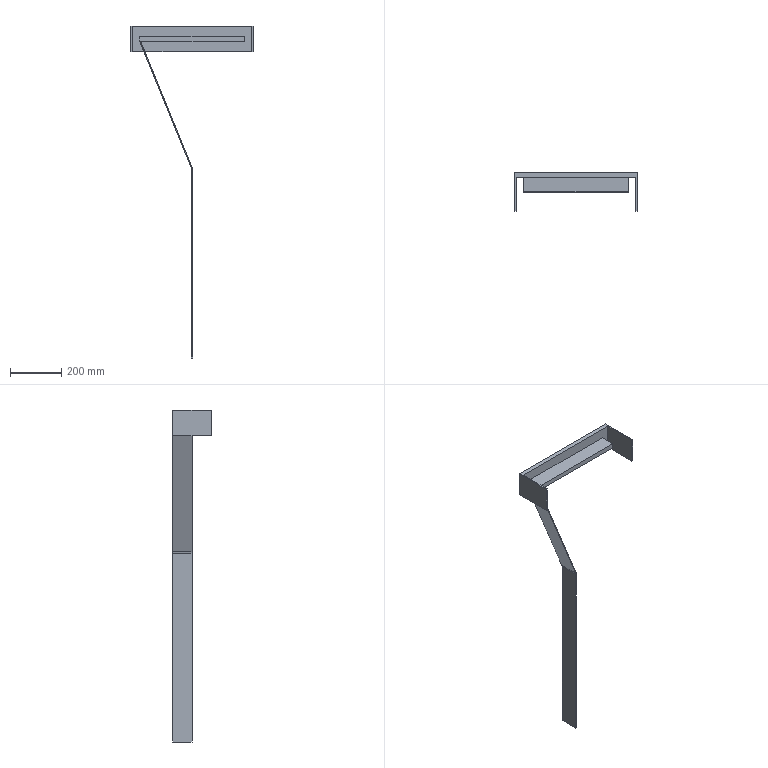Part | STEP file | Flat conveyor mechanism-Part11 | 1 solid | 25 faces | box 476 x 150 x 1294 mm | volume 1809742 mm3 | plane 23 | cylinder 2 | commonest cylinder face diameters 40 x2
STEP:
#1=CARTESIAN_POINT('',(-187.827,150.,0.));
#2=VERTEX_POINT('',#1);
#3=CARTESIAN_POINT('',(-238.,150.,0.));
#4=VERTEX_POINT('',#3);
#5=CARTESIAN_POINT('',(-233.,150.,0.));
#6=DIRECTION('',(-1.,0.,0.));
#7=VECTOR('',#6,1000.);
#8=LINE('',#5,#7);
#9=EDGE_CURVE('',#2,#4,#8,.T.);
#10=ORIENTED_EDGE('',*,*,#9,.F.);
#11=CARTESIAN_POINT('',(-187.827,132.31,0.));
#12=VERTEX_POINT('',#11);
#13=CARTESIAN_POINT('',(-187.827,150.,0.));
#14=DIRECTION('',(0.,-1.,0.));
#15=VECTOR('',#14,1000.);
#16=LINE('',#13,#15);
#17=EDGE_CURVE('',#2,#12,#16,.T.);
#18=ORIENTED_EDGE('',*,*,#17,.T.);
#19=CARTESIAN_POINT('',(-233.,132.31,0.));
#20=VERTEX_POINT('',#19);
#21=CARTESIAN_POINT('',(238.,132.31,0.));
#22=DIRECTION('',(1.,0.,0.));
#23=VECTOR('',#22,1000.);
#24=LINE('',#21,#23);
#25=EDGE_CURVE('',#20,#12,#24,.T.);
#26=ORIENTED_EDGE('',*,*,#25,.F.);
#27=CARTESIAN_POINT('',(-233.,0.,0.));
#28=VERTEX_POINT('',#27);
#29=CARTESIAN_POINT('',(-233.,150.,0.));
#30=DIRECTION('',(0.,-1.,0.));
#31=VECTOR('',#30,1000.);
#32=LINE('',#29,#31);
#33=EDGE_CURVE('',#20,#28,#32,.T.);
#34=ORIENTED_EDGE('',*,*,#33,.T.);
#35=CARTESIAN_POINT('',(-238.,0.,0.));
#36=VERTEX_POINT('',#35);
#37=CARTESIAN_POINT('',(-233.,0.,0.));
#38=DIRECTION('',(-1.,0.,0.));
#39=VECTOR('',#38,1000.);
#40=LINE('',#37,#39);
#41=EDGE_CURVE('',#28,#36,#40,.T.);
#42=ORIENTED_EDGE('',*,*,#41,.T.);
#43=CARTESIAN_POINT('',(-238.,150.,0.));
#44=DIRECTION('',(0.,-1.,0.));
#45=VECTOR('',#44,1000.);
#46=LINE('',#43,#45);
#47=EDGE_CURVE('',#4,#36,#46,.T.);
#48=ORIENTED_EDGE('',*,*,#47,.F.);
#49=EDGE_LOOP('',(#10,#18,#26,#34,#42,#48));
#50=FACE_OUTER_BOUND('',#49,.T.);
#51=CARTESIAN_POINT('',(-233.,150.,0.));
#52=DIRECTION('',(0.,0.,1.));
#53=DIRECTION('',(1.,0.,0.));
#54=AXIS2_PLACEMENT_3D('',#51,#52,#53);
#55=PLANE('',#54);
#56=ADVANCED_FACE('',(#50),#55,.F.);
#57=CARTESIAN_POINT('',(-204.,74.99,49.559));
#58=VERTEX_POINT('',#57);
#59=CARTESIAN_POINT('',(-204.,132.31,49.559));
#60=VERTEX_POINT('',#59);
#61=CARTESIAN_POINT('',(-204.,69.99,49.559));
#62=DIRECTION('',(0.,1.,0.));
#63=VECTOR('',#62,1000.);
#64=LINE('',#61,#63);
#65=EDGE_CURVE('',#58,#60,#64,.T.);
#66=ORIENTED_EDGE('',*,*,#65,.F.);
#67=CARTESIAN_POINT('',(-204.,74.99,60.));
#68=VERTEX_POINT('',#67);
#69=CARTESIAN_POINT('',(-204.,74.99,-447.));
#70=DIRECTION('',(0.,0.,1.));
#71=VECTOR('',#70,1000.);
#72=LINE('',#69,#71);
#73=EDGE_CURVE('',#58,#68,#72,.T.);
#74=ORIENTED_EDGE('',*,*,#73,.T.);
#75=CARTESIAN_POINT('',(-204.,132.31,60.));
#76=VERTEX_POINT('',#75);
#77=CARTESIAN_POINT('',(-204.,74.99,60.));
#78=DIRECTION('',(0.,-1.,0.));
#79=VECTOR('',#78,1000.);
#80=LINE('',#77,#79);
#81=EDGE_CURVE('',#76,#68,#80,.T.);
#82=ORIENTED_EDGE('',*,*,#81,.F.);
#83=CARTESIAN_POINT('',(-204.,132.31,0.));
#84=DIRECTION('',(0.,0.,-1.));
#85=VECTOR('',#84,1000.);
#86=LINE('',#83,#85);
#87=EDGE_CURVE('',#76,#60,#86,.T.);
#88=ORIENTED_EDGE('',*,*,#87,.T.);
#89=EDGE_LOOP('',(#66,#74,#82,#88));
#90=FACE_OUTER_BOUND('',#89,.T.);
#91=CARTESIAN_POINT('',(-204.,69.99,0.));
#92=DIRECTION('',(-1.,0.,0.));
#93=DIRECTION('',(0.,0.,1.));
#94=AXIS2_PLACEMENT_3D('',#91,#92,#93);
#95=PLANE('',#94);
#96=ADVANCED_FACE('',(#90),#95,.T.);
#97=CARTESIAN_POINT('',(204.,74.99,40.));
#98=VERTEX_POINT('',#97);
#99=CARTESIAN_POINT('',(204.,132.31,40.));
#100=VERTEX_POINT('',#99);
#101=CARTESIAN_POINT('',(204.,74.99,40.));
#102=DIRECTION('',(0.,1.,0.));
#103=VECTOR('',#102,1000.);
#104=LINE('',#101,#103);
#105=EDGE_CURVE('',#98,#100,#104,.T.);
#106=ORIENTED_EDGE('',*,*,#105,.T.);
#107=CARTESIAN_POINT('',(204.,132.31,60.));
#108=VERTEX_POINT('',#107);
#109=CARTESIAN_POINT('',(204.,132.31,0.));
#110=DIRECTION('',(0.,0.,-1.));
#111=VECTOR('',#110,1000.);
#112=LINE('',#109,#111);
#113=EDGE_CURVE('',#108,#100,#112,.T.);
#114=ORIENTED_EDGE('',*,*,#113,.F.);
#115=CARTESIAN_POINT('',(204.,74.99,60.));
#116=VERTEX_POINT('',#115);
#117=CARTESIAN_POINT('',(204.,74.99,60.));
#118=DIRECTION('',(0.,1.,0.));
#119=VECTOR('',#118,1000.);
#120=LINE('',#117,#119);
#121=EDGE_CURVE('',#116,#108,#120,.T.);
#122=ORIENTED_EDGE('',*,*,#121,.F.);
#123=CARTESIAN_POINT('',(204.,74.99,0.));
#124=DIRECTION('',(0.,0.,-1.));
#125=VECTOR('',#124,1000.);
#126=LINE('',#123,#125);
#127=EDGE_CURVE('',#116,#98,#126,.T.);
#128=ORIENTED_EDGE('',*,*,#127,.T.);
#129=EDGE_LOOP('',(#106,#114,#122,#128));
#130=FACE_OUTER_BOUND('',#129,.T.);
#131=CARTESIAN_POINT('',(204.,69.99,0.));
#132=DIRECTION('',(-1.,0.,0.));
#133=DIRECTION('',(0.,0.,1.));
#134=AXIS2_PLACEMENT_3D('',#131,#132,#133);
#135=PLANE('',#134);
#136=ADVANCED_FACE('',(#130),#135,.F.);
#137=CARTESIAN_POINT('',(2.,74.99,-460.437));
#138=VERTEX_POINT('',#137);
#139=CARTESIAN_POINT('',(2.,74.99,-1194.458));
#140=VERTEX_POINT('',#139);
#141=CARTESIAN_POINT('',(2.,74.99,-1194.458));
#142=DIRECTION('',(0.,0.,-1.));
#143=VECTOR('',#142,1000.);
#144=LINE('',#141,#143);
#145=EDGE_CURVE('',#138,#140,#144,.T.);
#146=ORIENTED_EDGE('',*,*,#145,.F.);
#147=CARTESIAN_POINT('',(0.5242,74.99,-452.897));
#148=VERTEX_POINT('',#147);
#149=CARTESIAN_POINT('',(-18.,74.99,-460.437));
#150=DIRECTION('',(0.,-1.,0.));
#151=DIRECTION('',(-1.,0.,0.));
#152=AXIS2_PLACEMENT_3D('',#149,#150,#151);
#153=CIRCLE('',#152,20.);
#154=EDGE_CURVE('',#138,#148,#153,.T.);
#155=ORIENTED_EDGE('',*,*,#154,.T.);
#156=CARTESIAN_POINT('',(-200.109,74.99,40.));
#157=VERTEX_POINT('',#156);
#158=CARTESIAN_POINT('',(2.,74.99,-456.522));
#159=DIRECTION('',(0.377,0.,-0.9262));
#160=VECTOR('',#159,1000.);
#161=LINE('',#158,#160);
#162=EDGE_CURVE('',#157,#148,#161,.T.);
#163=ORIENTED_EDGE('',*,*,#162,.F.);
#164=CARTESIAN_POINT('',(204.,74.99,40.));
#165=DIRECTION('',(1.,0.,0.));
#166=VECTOR('',#165,1000.);
#167=LINE('',#164,#166);
#168=EDGE_CURVE('',#157,#98,#167,.T.);
#169=ORIENTED_EDGE('',*,*,#168,.T.);
#170=ORIENTED_EDGE('',*,*,#127,.F.);
#171=CARTESIAN_POINT('',(204.,74.99,60.));
#172=DIRECTION('',(1.,0.,0.));
#173=VECTOR('',#172,1000.);
#174=LINE('',#171,#173);
#175=EDGE_CURVE('',#68,#116,#174,.T.);
#176=ORIENTED_EDGE('',*,*,#175,.F.);
#177=ORIENTED_EDGE('',*,*,#73,.F.);
#178=CARTESIAN_POINT('',(-204.179,74.99,50.));
#179=VERTEX_POINT('',#178);
#180=CARTESIAN_POINT('',(2.,74.99,-456.522));
#181=DIRECTION('',(0.377,0.,-0.9262));
#182=VECTOR('',#181,1000.);
#183=LINE('',#180,#182);
#184=EDGE_CURVE('',#179,#58,#183,.T.);
#185=ORIENTED_EDGE('',*,*,#184,.F.);
#186=CARTESIAN_POINT('',(-204.179,74.99,40.173));
#187=VERTEX_POINT('',#186);
#188=CARTESIAN_POINT('',(-204.179,74.99,40.173));
#189=DIRECTION('',(0.,0.,1.));
#190=VECTOR('',#189,1000.);
#191=LINE('',#188,#190);
#192=EDGE_CURVE('',#187,#179,#191,.T.);
#193=ORIENTED_EDGE('',*,*,#192,.F.);
#194=CARTESIAN_POINT('',(-3.476,74.99,-452.897));
#195=VERTEX_POINT('',#194);
#196=CARTESIAN_POINT('',(-2.,74.99,-456.522));
#197=DIRECTION('',(-0.377,0.,0.9262));
#198=VECTOR('',#197,1000.);
#199=LINE('',#196,#198);
#200=EDGE_CURVE('',#195,#187,#199,.T.);
#201=ORIENTED_EDGE('',*,*,#200,.F.);
#202=CARTESIAN_POINT('',(-2.,74.99,-460.437));
#203=VERTEX_POINT('',#202);
#204=CARTESIAN_POINT('',(-22.,74.99,-460.437));
#205=DIRECTION('',(0.,1.,0.));
#206=DIRECTION('',(-1.,0.,0.));
#207=AXIS2_PLACEMENT_3D('',#204,#205,#206);
#208=CIRCLE('',#207,20.);
#209=EDGE_CURVE('',#195,#203,#208,.T.);
#210=ORIENTED_EDGE('',*,*,#209,.T.);
#211=CARTESIAN_POINT('',(-2.,74.99,-1194.458));
#212=VERTEX_POINT('',#211);
#213=CARTESIAN_POINT('',(-2.,74.99,-1194.458));
#214=DIRECTION('',(0.,0.,1.));
#215=VECTOR('',#214,1000.);
#216=LINE('',#213,#215);
#217=EDGE_CURVE('',#212,#203,#216,.T.);
#218=ORIENTED_EDGE('',*,*,#217,.F.);
#219=CARTESIAN_POINT('',(2.,74.99,-1194.458));
#220=DIRECTION('',(-1.,0.,0.));
#221=VECTOR('',#220,1000.);
#222=LINE('',#219,#221);
#223=EDGE_CURVE('',#140,#212,#222,.T.);
#224=ORIENTED_EDGE('',*,*,#223,.F.);
#225=EDGE_LOOP('',(#146,#155,#163,#169,#170,#176,#177,#185,#193,#201,#210,#218,#224));
#226=FACE_OUTER_BOUND('',#225,.T.);
#227=CARTESIAN_POINT('',(204.,74.99,-447.));
#228=DIRECTION('',(0.,1.,0.));
#229=DIRECTION('',(-1.,0.,0.));
#230=AXIS2_PLACEMENT_3D('',#227,#228,#229);
#231=PLANE('',#230);
#232=ADVANCED_FACE('',(#226),#231,.F.);
#233=CARTESIAN_POINT('',(-183.827,132.31,0.));
#234=VERTEX_POINT('',#233);
#235=CARTESIAN_POINT('',(233.,132.31,0.));
#236=VERTEX_POINT('',#235);
#237=CARTESIAN_POINT('',(238.,132.31,0.));
#238=DIRECTION('',(1.,0.,0.));
#239=VECTOR('',#238,1000.);
#240=LINE('',#237,#239);
#241=EDGE_CURVE('',#234,#236,#240,.T.);
#242=ORIENTED_EDGE('',*,*,#241,.F.);
#243=CARTESIAN_POINT('',(-183.827,150.,0.));
#244=VERTEX_POINT('',#243);
#245=CARTESIAN_POINT('',(-183.827,150.,0.));
#246=DIRECTION('',(0.,1.,0.));
#247=VECTOR('',#246,1000.);
#248=LINE('',#245,#247);
#249=EDGE_CURVE('',#234,#244,#248,.T.);
#250=ORIENTED_EDGE('',*,*,#249,.T.);
#251=CARTESIAN_POINT('',(238.,150.,0.));
#252=VERTEX_POINT('',#251);
#253=CARTESIAN_POINT('',(-233.,150.,0.));
#254=DIRECTION('',(-1.,0.,0.));
#255=VECTOR('',#254,1000.);
#256=LINE('',#253,#255);
#257=EDGE_CURVE('',#252,#244,#256,.T.);
#258=ORIENTED_EDGE('',*,*,#257,.F.);
#259=CARTESIAN_POINT('',(238.,0.,0.));
#260=VERTEX_POINT('',#259);
#261=CARTESIAN_POINT('',(238.,150.,0.));
#262=DIRECTION('',(0.,1.,0.));
#263=VECTOR('',#262,1000.);
#264=LINE('',#261,#263);
#265=EDGE_CURVE('',#260,#252,#264,.T.);
#266=ORIENTED_EDGE('',*,*,#265,.F.);
#267=CARTESIAN_POINT('',(233.,0.,0.));
#268=VERTEX_POINT('',#267);
#269=CARTESIAN_POINT('',(233.,0.,0.));
#270=DIRECTION('',(-1.,0.,0.));
#271=VECTOR('',#270,1000.);
#272=LINE('',#269,#271);
#273=EDGE_CURVE('',#260,#268,#272,.T.);
#274=ORIENTED_EDGE('',*,*,#273,.T.);
#275=CARTESIAN_POINT('',(233.,150.,0.));
#276=DIRECTION('',(0.,-1.,0.));
#277=VECTOR('',#276,1000.);
#278=LINE('',#275,#277);
#279=EDGE_CURVE('',#236,#268,#278,.T.);
#280=ORIENTED_EDGE('',*,*,#279,.F.);
#281=EDGE_LOOP('',(#242,#250,#258,#266,#274,#280));
#282=FACE_OUTER_BOUND('',#281,.T.);
#283=CARTESIAN_POINT('',(-233.,150.,0.));
#284=DIRECTION('',(0.,0.,1.));
#285=DIRECTION('',(1.,0.,0.));
#286=AXIS2_PLACEMENT_3D('',#283,#284,#285);
#287=PLANE('',#286);
#288=ADVANCED_FACE('',(#282),#287,.F.);
#289=CARTESIAN_POINT('',(-200.109,132.31,40.));
#290=VERTEX_POINT('',#289);
#291=CARTESIAN_POINT('',(-124.083,132.31,-146.775));
#292=DIRECTION('',(-0.377,0.,0.9262));
#293=VECTOR('',#292,1000.);
#294=LINE('',#291,#293);
#295=EDGE_CURVE('',#234,#290,#294,.T.);
#296=ORIENTED_EDGE('',*,*,#295,.F.);
#297=ORIENTED_EDGE('',*,*,#241,.T.);
#298=CARTESIAN_POINT('',(233.,132.31,100.));
#299=VERTEX_POINT('',#298);
#300=CARTESIAN_POINT('',(233.,132.31,0.));
#301=DIRECTION('',(0.,0.,1.));
#302=VECTOR('',#301,1000.);
#303=LINE('',#300,#302);
#304=EDGE_CURVE('',#236,#299,#303,.T.);
#305=ORIENTED_EDGE('',*,*,#304,.T.);
#306=CARTESIAN_POINT('',(-233.,132.31,100.));
#307=VERTEX_POINT('',#306);
#308=CARTESIAN_POINT('',(236.5,132.31,100.));
#309=DIRECTION('',(1.,0.,0.));
#310=VECTOR('',#309,1000.);
#311=LINE('',#308,#310);
#312=EDGE_CURVE('',#307,#299,#311,.T.);
#313=ORIENTED_EDGE('',*,*,#312,.F.);
#314=CARTESIAN_POINT('',(-233.,132.31,0.));
#315=DIRECTION('',(0.,0.,1.));
#316=VECTOR('',#315,1000.);
#317=LINE('',#314,#316);
#318=EDGE_CURVE('',#20,#307,#317,.T.);
#319=ORIENTED_EDGE('',*,*,#318,.F.);
#320=ORIENTED_EDGE('',*,*,#25,.T.);
#321=CARTESIAN_POINT('',(-204.179,132.31,40.173));
#322=VERTEX_POINT('',#321);
#323=CARTESIAN_POINT('',(-127.514,132.31,-148.172));
#324=DIRECTION('',(0.377,0.,-0.9262));
#325=VECTOR('',#324,1000.);
#326=LINE('',#323,#325);
#327=EDGE_CURVE('',#322,#12,#326,.T.);
#328=ORIENTED_EDGE('',*,*,#327,.F.);
#329=CARTESIAN_POINT('',(-204.179,132.31,50.));
#330=VERTEX_POINT('',#329);
#331=CARTESIAN_POINT('',(-204.179,132.31,0.));
#332=DIRECTION('',(0.,0.,-1.));
#333=VECTOR('',#332,1000.);
#334=LINE('',#331,#333);
#335=EDGE_CURVE('',#330,#322,#334,.T.);
#336=ORIENTED_EDGE('',*,*,#335,.F.);
#337=CARTESIAN_POINT('',(-124.083,132.31,-146.775));
#338=DIRECTION('',(-0.377,0.,0.9262));
#339=VECTOR('',#338,1000.);
#340=LINE('',#337,#339);
#341=EDGE_CURVE('',#60,#330,#340,.T.);
#342=ORIENTED_EDGE('',*,*,#341,.F.);
#343=ORIENTED_EDGE('',*,*,#87,.F.);
#344=CARTESIAN_POINT('',(204.,132.31,60.));
#345=DIRECTION('',(-1.,0.,0.));
#346=VECTOR('',#345,1000.);
#347=LINE('',#344,#346);
#348=EDGE_CURVE('',#108,#76,#347,.T.);
#349=ORIENTED_EDGE('',*,*,#348,.F.);
#350=ORIENTED_EDGE('',*,*,#113,.T.);
#351=CARTESIAN_POINT('',(204.,132.31,40.));
#352=DIRECTION('',(-1.,0.,0.));
#353=VECTOR('',#352,1000.);
#354=LINE('',#351,#353);
#355=EDGE_CURVE('',#100,#290,#354,.T.);
#356=ORIENTED_EDGE('',*,*,#355,.T.);
#357=EDGE_LOOP('',(#296,#297,#305,#313,#319,#320,#328,#336,#342,#343,#349,#350,#356));
#358=FACE_OUTER_BOUND('',#357,.T.);
#359=CARTESIAN_POINT('',(236.5,132.31,0.));
#360=DIRECTION('',(0.,-1.,0.));
#361=DIRECTION('',(1.,0.,0.));
#362=AXIS2_PLACEMENT_3D('',#359,#360,#361);
#363=PLANE('',#362);
#364=ADVANCED_FACE('',(#358),#363,.T.);
#365=ORIENTED_EDGE('',*,*,#33,.F.);
#366=ORIENTED_EDGE('',*,*,#318,.T.);
#367=CARTESIAN_POINT('',(-233.,0.,100.));
#368=VERTEX_POINT('',#367);
#369=CARTESIAN_POINT('',(-233.,150.,100.));
#370=DIRECTION('',(0.,-1.,0.));
#371=VECTOR('',#370,1000.);
#372=LINE('',#369,#371);
#373=EDGE_CURVE('',#307,#368,#372,.T.);
#374=ORIENTED_EDGE('',*,*,#373,.T.);
#375=CARTESIAN_POINT('',(-233.,0.,0.));
#376=DIRECTION('',(0.,0.,-1.));
#377=VECTOR('',#376,1000.);
#378=LINE('',#375,#377);
#379=EDGE_CURVE('',#368,#28,#378,.T.);
#380=ORIENTED_EDGE('',*,*,#379,.T.);
#381=EDGE_LOOP('',(#365,#366,#374,#380));
#382=FACE_OUTER_BOUND('',#381,.T.);
#383=CARTESIAN_POINT('',(-233.,150.,0.));
#384=DIRECTION('',(-1.,0.,0.));
#385=DIRECTION('',(0.,0.,1.));
#386=AXIS2_PLACEMENT_3D('',#383,#384,#385);
#387=PLANE('',#386);
#388=ADVANCED_FACE('',(#382),#387,.F.);
#389=CARTESIAN_POINT('',(-238.,0.,100.));
#390=VERTEX_POINT('',#389);
#391=CARTESIAN_POINT('',(-238.,0.,0.));
#392=DIRECTION('',(0.,0.,1.));
#393=VECTOR('',#392,1000.);
#394=LINE('',#391,#393);
#395=EDGE_CURVE('',#36,#390,#394,.T.);
#396=ORIENTED_EDGE('',*,*,#395,.T.);
#397=CARTESIAN_POINT('',(-238.,150.,100.));
#398=VERTEX_POINT('',#397);
#399=CARTESIAN_POINT('',(-238.,150.,100.));
#400=DIRECTION('',(0.,-1.,0.));
#401=VECTOR('',#400,1000.);
#402=LINE('',#399,#401);
#403=EDGE_CURVE('',#398,#390,#402,.T.);
#404=ORIENTED_EDGE('',*,*,#403,.F.);
#405=CARTESIAN_POINT('',(-238.,150.,0.));
#406=DIRECTION('',(0.,0.,1.));
#407=VECTOR('',#406,1000.);
#408=LINE('',#405,#407);
#409=EDGE_CURVE('',#4,#398,#408,.T.);
#410=ORIENTED_EDGE('',*,*,#409,.F.);
#411=ORIENTED_EDGE('',*,*,#47,.T.);
#412=EDGE_LOOP('',(#396,#404,#410,#411));
#413=FACE_OUTER_BOUND('',#412,.T.);
#414=CARTESIAN_POINT('',(-238.,150.,0.));
#415=DIRECTION('',(1.,0.,0.));
#416=DIRECTION('',(0.,0.,-1.));
#417=AXIS2_PLACEMENT_3D('',#414,#415,#416);
#418=PLANE('',#417);
#419=ADVANCED_FACE('',(#413),#418,.F.);
#420=ORIENTED_EDGE('',*,*,#312,.T.);
#421=CARTESIAN_POINT('',(233.,0.,100.));
#422=VERTEX_POINT('',#421);
#423=CARTESIAN_POINT('',(233.,150.,100.));
#424=DIRECTION('',(0.,-1.,0.));
#425=VECTOR('',#424,1000.);
#426=LINE('',#423,#425);
#427=EDGE_CURVE('',#299,#422,#426,.T.);
#428=ORIENTED_EDGE('',*,*,#427,.T.);
#429=CARTESIAN_POINT('',(238.,0.,100.));
#430=VERTEX_POINT('',#429);
#431=CARTESIAN_POINT('',(233.,0.,100.));
#432=DIRECTION('',(1.,0.,0.));
#433=VECTOR('',#432,1000.);
#434=LINE('',#431,#433);
#435=EDGE_CURVE('',#422,#430,#434,.T.);
#436=ORIENTED_EDGE('',*,*,#435,.T.);
#437=CARTESIAN_POINT('',(238.,150.,100.));
#438=VERTEX_POINT('',#437);
#439=CARTESIAN_POINT('',(238.,150.,100.));
#440=DIRECTION('',(0.,1.,0.));
#441=VECTOR('',#440,1000.);
#442=LINE('',#439,#441);
#443=EDGE_CURVE('',#430,#438,#442,.T.);
#444=ORIENTED_EDGE('',*,*,#443,.T.);
#445=CARTESIAN_POINT('',(-233.,150.,100.));
#446=DIRECTION('',(1.,0.,0.));
#447=VECTOR('',#446,1000.);
#448=LINE('',#445,#447);
#449=EDGE_CURVE('',#398,#438,#448,.T.);
#450=ORIENTED_EDGE('',*,*,#449,.F.);
#451=ORIENTED_EDGE('',*,*,#403,.T.);
#452=CARTESIAN_POINT('',(-233.,0.,100.));
#453=DIRECTION('',(1.,0.,0.));
#454=VECTOR('',#453,1000.);
#455=LINE('',#452,#454);
#456=EDGE_CURVE('',#390,#368,#455,.T.);
#457=ORIENTED_EDGE('',*,*,#456,.T.);
#458=ORIENTED_EDGE('',*,*,#373,.F.);
#459=EDGE_LOOP('',(#420,#428,#436,#444,#450,#451,#457,#458));
#460=FACE_OUTER_BOUND('',#459,.T.);
#461=CARTESIAN_POINT('',(-233.,150.,100.));
#462=DIRECTION('',(0.,0.,-1.));
#463=DIRECTION('',(-1.,0.,0.));
#464=AXIS2_PLACEMENT_3D('',#461,#462,#463);
#465=PLANE('',#464);
#466=ADVANCED_FACE('',(#460),#465,.F.);
#467=CARTESIAN_POINT('',(0.5242,150.,-452.897));
#468=VERTEX_POINT('',#467);
#469=CARTESIAN_POINT('',(2.,150.,-456.522));
#470=DIRECTION('',(0.377,0.,-0.9262));
#471=VECTOR('',#470,1000.);
#472=LINE('',#469,#471);
#473=EDGE_CURVE('',#244,#468,#472,.T.);
#474=ORIENTED_EDGE('',*,*,#473,.T.);
#475=CARTESIAN_POINT('',(2.,150.,-460.437));
#476=VERTEX_POINT('',#475);
#477=CARTESIAN_POINT('',(-18.,150.,-460.437));
#478=DIRECTION('',(0.,1.,0.));
#479=DIRECTION('',(0.,0.,-1.));
#480=AXIS2_PLACEMENT_3D('',#477,#478,#479);
#481=CIRCLE('',#480,20.);
#482=EDGE_CURVE('',#468,#476,#481,.T.);
#483=ORIENTED_EDGE('',*,*,#482,.T.);
#484=CARTESIAN_POINT('',(2.,150.,-1194.458));
#485=VERTEX_POINT('',#484);
#486=CARTESIAN_POINT('',(2.,150.,-1194.458));
#487=DIRECTION('',(0.,0.,-1.));
#488=VECTOR('',#487,1000.);
#489=LINE('',#486,#488);
#490=EDGE_CURVE('',#476,#485,#489,.T.);
#491=ORIENTED_EDGE('',*,*,#490,.T.);
#492=CARTESIAN_POINT('',(-2.,150.,-1194.458));
#493=VERTEX_POINT('',#492);
#494=CARTESIAN_POINT('',(2.,150.,-1194.458));
#495=DIRECTION('',(-1.,0.,0.));
#496=VECTOR('',#495,1000.);
#497=LINE('',#494,#496);
#498=EDGE_CURVE('',#485,#493,#497,.T.);
#499=ORIENTED_EDGE('',*,*,#498,.T.);
#500=CARTESIAN_POINT('',(-2.,150.,-460.437));
#501=VERTEX_POINT('',#500);
#502=CARTESIAN_POINT('',(-2.,150.,-1194.458));
#503=DIRECTION('',(0.,0.,1.));
#504=VECTOR('',#503,1000.);
#505=LINE('',#502,#504);
#506=EDGE_CURVE('',#493,#501,#505,.T.);
#507=ORIENTED_EDGE('',*,*,#506,.T.);
#508=CARTESIAN_POINT('',(-3.476,150.,-452.897));
#509=VERTEX_POINT('',#508);
#510=CARTESIAN_POINT('',(-22.,150.,-460.437));
#511=DIRECTION('',(0.,-1.,0.));
#512=DIRECTION('',(0.,0.,-1.));
#513=AXIS2_PLACEMENT_3D('',#510,#511,#512);
#514=CIRCLE('',#513,20.);
#515=EDGE_CURVE('',#501,#509,#514,.T.);
#516=ORIENTED_EDGE('',*,*,#515,.T.);
#517=CARTESIAN_POINT('',(-2.,150.,-456.522));
#518=DIRECTION('',(-0.377,0.,0.9262));
#519=VECTOR('',#518,1000.);
#520=LINE('',#517,#519);
#521=EDGE_CURVE('',#509,#2,#520,.T.);
#522=ORIENTED_EDGE('',*,*,#521,.T.);
#523=ORIENTED_EDGE('',*,*,#9,.T.);
#524=ORIENTED_EDGE('',*,*,#409,.T.);
#525=ORIENTED_EDGE('',*,*,#449,.T.);
#526=CARTESIAN_POINT('',(238.,150.,0.));
#527=DIRECTION('',(0.,0.,1.));
#528=VECTOR('',#527,1000.);
#529=LINE('',#526,#528);
#530=EDGE_CURVE('',#252,#438,#529,.T.);
#531=ORIENTED_EDGE('',*,*,#530,.F.);
#532=ORIENTED_EDGE('',*,*,#257,.T.);
#533=EDGE_LOOP('',(#474,#483,#491,#499,#507,#516,#522,#523,#524,#525,#531,#532));
#534=FACE_OUTER_BOUND('',#533,.T.);
#535=CARTESIAN_POINT('',(0.,150.,0.));
#536=DIRECTION('',(0.,-1.,0.));
#537=DIRECTION('',(0.,0.,-1.));
#538=AXIS2_PLACEMENT_3D('',#535,#536,#537);
#539=PLANE('',#538);
#540=ADVANCED_FACE('',(#534),#539,.F.);
#541=ORIENTED_EDGE('',*,*,#379,.F.);
#542=ORIENTED_EDGE('',*,*,#456,.F.);
#543=ORIENTED_EDGE('',*,*,#395,.F.);
#544=ORIENTED_EDGE('',*,*,#41,.F.);
#545=EDGE_LOOP('',(#541,#542,#543,#544));
#546=FACE_OUTER_BOUND('',#545,.T.);
#547=CARTESIAN_POINT('',(0.,0.,0.));
#548=DIRECTION('',(0.,-1.,0.));
#549=DIRECTION('',(0.,0.,-1.));
#550=AXIS2_PLACEMENT_3D('',#547,#548,#549);
#551=PLANE('',#550);
#552=ADVANCED_FACE('',(#546),#551,.T.);
#553=ORIENTED_EDGE('',*,*,#443,.F.);
#554=CARTESIAN_POINT('',(238.,0.,0.));
#555=DIRECTION('',(0.,0.,-1.));
#556=VECTOR('',#555,1000.);
#557=LINE('',#554,#556);
#558=EDGE_CURVE('',#430,#260,#557,.T.);
#559=ORIENTED_EDGE('',*,*,#558,.T.);
#560=ORIENTED_EDGE('',*,*,#265,.T.);
#561=ORIENTED_EDGE('',*,*,#530,.T.);
#562=EDGE_LOOP('',(#553,#559,#560,#561));
#563=FACE_OUTER_BOUND('',#562,.T.);
#564=CARTESIAN_POINT('',(238.,150.,0.));
#565=DIRECTION('',(1.,0.,0.));
#566=DIRECTION('',(0.,0.,-1.));
#567=AXIS2_PLACEMENT_3D('',#564,#565,#566);
#568=PLANE('',#567);
#569=ADVANCED_FACE('',(#563),#568,.T.);
#570=ORIENTED_EDGE('',*,*,#304,.F.);
#571=ORIENTED_EDGE('',*,*,#279,.T.);
#572=CARTESIAN_POINT('',(233.,0.,0.));
#573=DIRECTION('',(0.,0.,1.));
#574=VECTOR('',#573,1000.);
#575=LINE('',#572,#574);
#576=EDGE_CURVE('',#268,#422,#575,.T.);
#577=ORIENTED_EDGE('',*,*,#576,.T.);
#578=ORIENTED_EDGE('',*,*,#427,.F.);
#579=EDGE_LOOP('',(#570,#571,#577,#578));
#580=FACE_OUTER_BOUND('',#579,.T.);
#581=CARTESIAN_POINT('',(233.,150.,0.));
#582=DIRECTION('',(1.,0.,0.));
#583=DIRECTION('',(0.,0.,-1.));
#584=AXIS2_PLACEMENT_3D('',#581,#582,#583);
#585=PLANE('',#584);
#586=ADVANCED_FACE('',(#580),#585,.F.);
#587=ORIENTED_EDGE('',*,*,#576,.F.);
#588=ORIENTED_EDGE('',*,*,#273,.F.);
#589=ORIENTED_EDGE('',*,*,#558,.F.);
#590=ORIENTED_EDGE('',*,*,#435,.F.);
#591=EDGE_LOOP('',(#587,#588,#589,#590));
#592=FACE_OUTER_BOUND('',#591,.T.);
#593=CARTESIAN_POINT('',(0.,0.,0.));
#594=DIRECTION('',(0.,1.,0.));
#595=DIRECTION('',(0.,0.,1.));
#596=AXIS2_PLACEMENT_3D('',#593,#594,#595);
#597=PLANE('',#596);
#598=ADVANCED_FACE('',(#592),#597,.F.);
#599=ORIENTED_EDGE('',*,*,#121,.T.);
#600=ORIENTED_EDGE('',*,*,#348,.T.);
#601=ORIENTED_EDGE('',*,*,#81,.T.);
#602=ORIENTED_EDGE('',*,*,#175,.T.);
#603=EDGE_LOOP('',(#599,#600,#601,#602));
#604=FACE_OUTER_BOUND('',#603,.T.);
#605=CARTESIAN_POINT('',(0.,0.,60.));
#606=DIRECTION('',(0.,0.,1.));
#607=DIRECTION('',(1.,0.,0.));
#608=AXIS2_PLACEMENT_3D('',#605,#606,#607);
#609=PLANE('',#608);
#610=ADVANCED_FACE('',(#604),#609,.T.);
#611=CARTESIAN_POINT('',(-200.109,0.,40.));
#612=DIRECTION('',(0.,-1.,0.));
#613=VECTOR('',#612,1000.);
#614=LINE('',#611,#613);
#615=EDGE_CURVE('',#290,#157,#614,.T.);
#616=ORIENTED_EDGE('',*,*,#615,.F.);
#617=ORIENTED_EDGE('',*,*,#355,.F.);
#618=ORIENTED_EDGE('',*,*,#105,.F.);
#619=ORIENTED_EDGE('',*,*,#168,.F.);
#620=EDGE_LOOP('',(#616,#617,#618,#619));
#621=FACE_OUTER_BOUND('',#620,.T.);
#622=CARTESIAN_POINT('',(0.,0.,40.));
#623=DIRECTION('',(0.,0.,-1.));
#624=DIRECTION('',(1.,0.,0.));
#625=AXIS2_PLACEMENT_3D('',#622,#623,#624);
#626=PLANE('',#625);
#627=ADVANCED_FACE('',(#621),#626,.T.);
#628=ORIENTED_EDGE('',*,*,#521,.F.);
#629=CARTESIAN_POINT('',(-3.476,74.99,-452.897));
#630=DIRECTION('',(0.,-1.,0.));
#631=VECTOR('',#630,1000.);
#632=LINE('',#629,#631);
#633=EDGE_CURVE('',#509,#195,#632,.T.);
#634=ORIENTED_EDGE('',*,*,#633,.T.);
#635=ORIENTED_EDGE('',*,*,#200,.T.);
#636=CARTESIAN_POINT('',(-204.179,74.99,40.173));
#637=DIRECTION('',(0.,1.,0.));
#638=VECTOR('',#637,1000.);
#639=LINE('',#636,#638);
#640=EDGE_CURVE('',#187,#322,#639,.T.);
#641=ORIENTED_EDGE('',*,*,#640,.T.);
#642=ORIENTED_EDGE('',*,*,#327,.T.);
#643=ORIENTED_EDGE('',*,*,#17,.F.);
#644=EDGE_LOOP('',(#628,#634,#635,#641,#642,#643));
#645=FACE_OUTER_BOUND('',#644,.T.);
#646=CARTESIAN_POINT('',(-2.,74.99,-456.522));
#647=DIRECTION('',(-0.9262,0.,-0.377));
#648=DIRECTION('',(-0.377,0.,0.9262));
#649=AXIS2_PLACEMENT_3D('',#646,#647,#648);
#650=PLANE('',#649);
#651=ADVANCED_FACE('',(#645),#650,.T.);
#652=ORIENTED_EDGE('',*,*,#162,.T.);
#653=CARTESIAN_POINT('',(0.5242,74.99,-452.897));
#654=DIRECTION('',(0.,1.,0.));
#655=VECTOR('',#654,1000.);
#656=LINE('',#653,#655);
#657=EDGE_CURVE('',#148,#468,#656,.T.);
#658=ORIENTED_EDGE('',*,*,#657,.T.);
#659=ORIENTED_EDGE('',*,*,#473,.F.);
#660=ORIENTED_EDGE('',*,*,#249,.F.);
#661=ORIENTED_EDGE('',*,*,#295,.T.);
#662=ORIENTED_EDGE('',*,*,#615,.T.);
#663=EDGE_LOOP('',(#652,#658,#659,#660,#661,#662));
#664=FACE_OUTER_BOUND('',#663,.T.);
#665=CARTESIAN_POINT('',(2.,74.99,-456.522));
#666=DIRECTION('',(0.9262,0.,0.377));
#667=DIRECTION('',(0.377,0.,-0.9262));
#668=AXIS2_PLACEMENT_3D('',#665,#666,#667);
#669=PLANE('',#668);
#670=ADVANCED_FACE('',(#664),#669,.T.);
#671=ORIENTED_EDGE('',*,*,#217,.T.);
#672=CARTESIAN_POINT('',(-2.,150.,-460.437));
#673=DIRECTION('',(0.,1.,0.));
#674=VECTOR('',#673,1000.);
#675=LINE('',#672,#674);
#676=EDGE_CURVE('',#203,#501,#675,.T.);
#677=ORIENTED_EDGE('',*,*,#676,.T.);
#678=ORIENTED_EDGE('',*,*,#506,.F.);
#679=CARTESIAN_POINT('',(-2.,74.99,-1194.458));
#680=DIRECTION('',(0.,1.,0.));
#681=VECTOR('',#680,1000.);
#682=LINE('',#679,#681);
#683=EDGE_CURVE('',#212,#493,#682,.T.);
#684=ORIENTED_EDGE('',*,*,#683,.F.);
#685=EDGE_LOOP('',(#671,#677,#678,#684));
#686=FACE_OUTER_BOUND('',#685,.T.);
#687=CARTESIAN_POINT('',(-2.,74.99,-1194.458));
#688=DIRECTION('',(-1.,0.,0.));
#689=DIRECTION('',(0.,0.,1.));
#690=AXIS2_PLACEMENT_3D('',#687,#688,#689);
#691=PLANE('',#690);
#692=ADVANCED_FACE('',(#686),#691,.T.);
#693=ORIENTED_EDGE('',*,*,#498,.F.);
#694=CARTESIAN_POINT('',(2.,74.99,-1194.458));
#695=DIRECTION('',(0.,1.,0.));
#696=VECTOR('',#695,1000.);
#697=LINE('',#694,#696);
#698=EDGE_CURVE('',#140,#485,#697,.T.);
#699=ORIENTED_EDGE('',*,*,#698,.F.);
#700=ORIENTED_EDGE('',*,*,#223,.T.);
#701=ORIENTED_EDGE('',*,*,#683,.T.);
#702=EDGE_LOOP('',(#693,#699,#700,#701));
#703=FACE_OUTER_BOUND('',#702,.T.);
#704=CARTESIAN_POINT('',(2.,74.99,-1194.458));
#705=DIRECTION('',(0.,0.,-1.));
#706=DIRECTION('',(-1.,0.,0.));
#707=AXIS2_PLACEMENT_3D('',#704,#705,#706);
#708=PLANE('',#707);
#709=ADVANCED_FACE('',(#703),#708,.T.);
#710=ORIENTED_EDGE('',*,*,#490,.F.);
#711=CARTESIAN_POINT('',(2.,74.99,-460.437));
#712=DIRECTION('',(0.,-1.,0.));
#713=VECTOR('',#712,1000.);
#714=LINE('',#711,#713);
#715=EDGE_CURVE('',#476,#138,#714,.T.);
#716=ORIENTED_EDGE('',*,*,#715,.T.);
#717=ORIENTED_EDGE('',*,*,#145,.T.);
#718=ORIENTED_EDGE('',*,*,#698,.T.);
#719=EDGE_LOOP('',(#710,#716,#717,#718));
#720=FACE_OUTER_BOUND('',#719,.T.);
#721=CARTESIAN_POINT('',(2.,74.99,-1194.458));
#722=DIRECTION('',(1.,0.,0.));
#723=DIRECTION('',(0.,0.,-1.));
#724=AXIS2_PLACEMENT_3D('',#721,#722,#723);
#725=PLANE('',#724);
#726=ADVANCED_FACE('',(#720),#725,.T.);
#727=ORIENTED_EDGE('',*,*,#184,.T.);
#728=ORIENTED_EDGE('',*,*,#65,.T.);
#729=ORIENTED_EDGE('',*,*,#341,.T.);
#730=CARTESIAN_POINT('',(-204.179,74.99,50.));
#731=DIRECTION('',(0.,1.,0.));
#732=VECTOR('',#731,1000.);
#733=LINE('',#730,#732);
#734=EDGE_CURVE('',#179,#330,#733,.T.);
#735=ORIENTED_EDGE('',*,*,#734,.F.);
#736=EDGE_LOOP('',(#727,#728,#729,#735));
#737=FACE_OUTER_BOUND('',#736,.T.);
#738=CARTESIAN_POINT('',(2.,74.99,-456.522));
#739=DIRECTION('',(0.9262,0.,0.377));
#740=DIRECTION('',(0.377,0.,-0.9262));
#741=AXIS2_PLACEMENT_3D('',#738,#739,#740);
#742=PLANE('',#741);
#743=ADVANCED_FACE('',(#737),#742,.T.);
#744=ORIENTED_EDGE('',*,*,#734,.T.);
#745=ORIENTED_EDGE('',*,*,#335,.T.);
#746=ORIENTED_EDGE('',*,*,#640,.F.);
#747=ORIENTED_EDGE('',*,*,#192,.T.);
#748=EDGE_LOOP('',(#744,#745,#746,#747));
#749=FACE_OUTER_BOUND('',#748,.T.);
#750=CARTESIAN_POINT('',(-204.179,74.99,40.173));
#751=DIRECTION('',(-1.,0.,0.));
#752=DIRECTION('',(0.,0.,1.));
#753=AXIS2_PLACEMENT_3D('',#750,#751,#752);
#754=PLANE('',#753);
#755=ADVANCED_FACE('',(#749),#754,.T.);
#756=ORIENTED_EDGE('',*,*,#209,.F.);
#757=ORIENTED_EDGE('',*,*,#633,.F.);
#758=ORIENTED_EDGE('',*,*,#515,.F.);
#759=ORIENTED_EDGE('',*,*,#676,.F.);
#760=EDGE_LOOP('',(#756,#757,#758,#759));
#761=FACE_OUTER_BOUND('',#760,.T.);
#762=CARTESIAN_POINT('',(-22.,74.99,-460.437));
#763=DIRECTION('',(0.,-1.,0.));
#764=DIRECTION('',(0.,0.,-1.));
#765=AXIS2_PLACEMENT_3D('',#762,#763,#764);
#766=CYLINDRICAL_SURFACE('',#765,20.);
#767=ADVANCED_FACE('',(#761),#766,.F.);
#768=ORIENTED_EDGE('',*,*,#154,.F.);
#769=ORIENTED_EDGE('',*,*,#715,.F.);
#770=ORIENTED_EDGE('',*,*,#482,.F.);
#771=ORIENTED_EDGE('',*,*,#657,.F.);
#772=EDGE_LOOP('',(#768,#769,#770,#771));
#773=FACE_OUTER_BOUND('',#772,.T.);
#774=CARTESIAN_POINT('',(-18.,74.99,-460.437));
#775=DIRECTION('',(0.,1.,0.));
#776=DIRECTION('',(0.,0.,1.));
#777=AXIS2_PLACEMENT_3D('',#774,#775,#776);
#778=CYLINDRICAL_SURFACE('',#777,20.);
#779=ADVANCED_FACE('',(#773),#778,.T.);
#780=CLOSED_SHELL('',(#56,#96,#136,#232,#288,#364,#388,#419,#466,#540,#552,#569,#586,#598,#610,#627,#651,#670,#692,#709,#726,#743,#755,#767,#779));
#781=MANIFOLD_SOLID_BREP('',#780);
#782=CARTESIAN_POINT('',(0.,0.,0.));
#783=DIRECTION('',(0.,0.,1.));
#784=DIRECTION('',(1.,0.,0.));
#785=AXIS2_PLACEMENT_3D('',#782,#783,#784);
#786=(LENGTH_UNIT()NAMED_UNIT(*)SI_UNIT(.MILLI.,.METRE.));
#787=UNCERTAINTY_MEASURE_WITH_UNIT(LENGTH_MEASURE(0.00001),#786,'','');
#788=(NAMED_UNIT(*)PLANE_ANGLE_UNIT()SI_UNIT($,.RADIAN.));
#789=(NAMED_UNIT(*)SI_UNIT($,.STERADIAN.)SOLID_ANGLE_UNIT());
#790=(GEOMETRIC_REPRESENTATION_CONTEXT(3)GLOBAL_UNCERTAINTY_ASSIGNED_CONTEXT((#787))GLOBAL_UNIT_ASSIGNED_CONTEXT((#786,#788,#789))REPRESENTATION_CONTEXT('',''));
#791=ADVANCED_BREP_SHAPE_REPRESENTATION('',(#781,#785),#790);